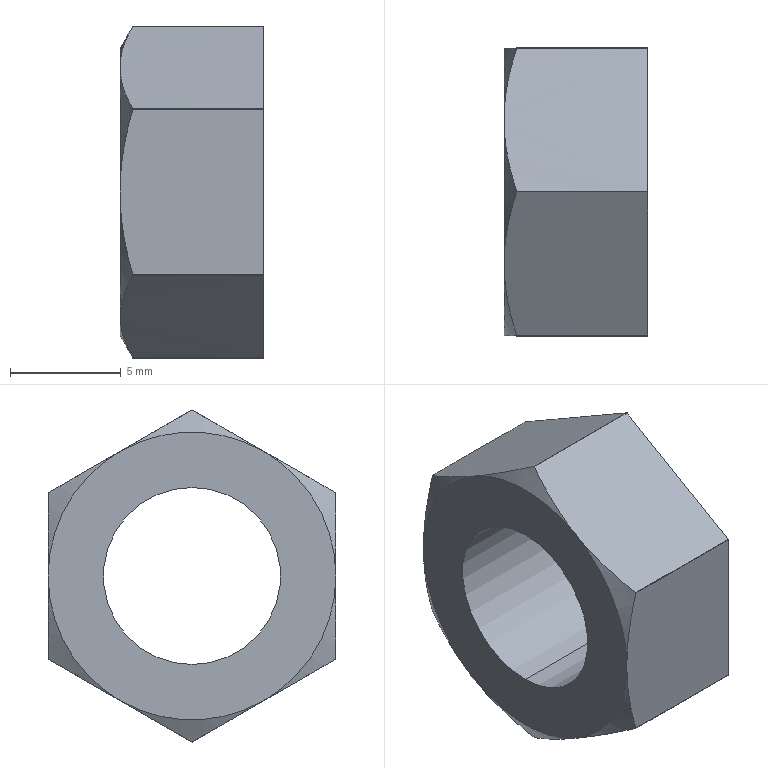Part | STEP file | TNSN20-Y20-F22-Part-12-1 | 1 solid | 22 faces | box 6.5 x 13.002 x 15 mm | volume 622.202 mm3 | cylinder 8 | plane 8 | cone 6 | commonest cylinder face diameters 15 x6 8 x2
STEP:
#1=CARTESIAN_POINT('',(14033.745,13720.046,23.));
#2=VERTEX_POINT('',#1);
#3=CARTESIAN_POINT('',(14033.745,13720.046,15.));
#4=VERTEX_POINT('',#3);
#5=CARTESIAN_POINT('',(14033.745,13720.046,19.));
#6=DIRECTION('',(1.,0.,0.));
#7=DIRECTION('',(0.,1.,0.));
#8=AXIS2_PLACEMENT_3D('',#5,#6,#7);
#9=CIRCLE('',#8,4.);
#10=EDGE_CURVE('',#2,#4,#9,.T.);
#11=ORIENTED_EDGE('',*,*,#10,.T.);
#12=CARTESIAN_POINT('',(14027.245,13720.046,15.));
#13=VERTEX_POINT('',#12);
#14=CARTESIAN_POINT('',(14036.245,13720.046,15.));
#15=DIRECTION('',(-1.,0.,0.));
#16=VECTOR('',#15,1000.);
#17=LINE('',#14,#16);
#18=EDGE_CURVE('',#4,#13,#17,.T.);
#19=ORIENTED_EDGE('',*,*,#18,.T.);
#20=CARTESIAN_POINT('',(14027.245,13720.046,23.));
#21=VERTEX_POINT('',#20);
#22=CARTESIAN_POINT('',(14027.245,13720.046,19.));
#23=DIRECTION('',(1.,0.,0.));
#24=DIRECTION('',(0.,1.,0.));
#25=AXIS2_PLACEMENT_3D('',#22,#23,#24);
#26=CIRCLE('',#25,4.);
#27=EDGE_CURVE('',#21,#13,#26,.T.);
#28=ORIENTED_EDGE('',*,*,#27,.F.);
#29=CARTESIAN_POINT('',(14036.245,13720.046,23.));
#30=DIRECTION('',(-1.,0.,0.));
#31=VECTOR('',#30,1000.);
#32=LINE('',#29,#31);
#33=EDGE_CURVE('',#2,#21,#32,.T.);
#34=ORIENTED_EDGE('',*,*,#33,.F.);
#35=EDGE_LOOP('',(#11,#19,#28,#34));
#36=FACE_OUTER_BOUND('',#35,.T.);
#37=CARTESIAN_POINT('',(14036.245,13720.046,19.));
#38=DIRECTION('',(-1.,0.,0.));
#39=DIRECTION('',(0.,0.,1.));
#40=AXIS2_PLACEMENT_3D('',#37,#38,#39);
#41=CYLINDRICAL_SURFACE('',#40,4.);
#42=ADVANCED_FACE('',(#36),#41,.F.);
#43=CARTESIAN_POINT('',(14027.822,13713.546,15.258));
#44=VERTEX_POINT('',#43);
#45=CARTESIAN_POINT('',(14027.822,13713.556,15.242));
#46=VERTEX_POINT('',#45);
#47=CARTESIAN_POINT('',(14027.822,13720.046,19.));
#48=DIRECTION('',(1.,0.,0.));
#49=DIRECTION('',(0.,-0.8667,-0.4989));
#50=AXIS2_PLACEMENT_3D('',#47,#48,#49);
#51=CIRCLE('',#50,7.5);
#52=EDGE_CURVE('',#44,#46,#51,.T.);
#53=ORIENTED_EDGE('',*,*,#52,.F.);
#54=CARTESIAN_POINT('',(14027.245,13713.546,19.));
#55=VERTEX_POINT('',#54);
#56=CARTESIAN_POINT('',(14027.822,13713.546,15.258));
#57=CARTESIAN_POINT('',(14027.647,13713.551,15.861));
#58=CARTESIAN_POINT('',(14027.502,13713.545,16.485));
#59=CARTESIAN_POINT('',(14027.3,13713.545,17.735));
#60=CARTESIAN_POINT('',(14027.244,13713.549,18.361));
#61=CARTESIAN_POINT('',(14027.245,13713.546,19.));
#62=B_SPLINE_CURVE_WITH_KNOTS('',3,(#56,#57,#58,#59,#60,#61),.UNSPECIFIED.,.F.,.F.,(4,2,4),(0.,0.5,1.),.UNSPECIFIED.);
#63=EDGE_CURVE('',#44,#55,#62,.T.);
#64=ORIENTED_EDGE('',*,*,#63,.T.);
#65=CARTESIAN_POINT('',(14027.245,13716.796,13.371));
#66=VERTEX_POINT('',#65);
#67=CARTESIAN_POINT('',(14027.245,13720.046,19.));
#68=DIRECTION('',(1.,0.,0.));
#69=DIRECTION('',(0.,-1.,0.));
#70=AXIS2_PLACEMENT_3D('',#67,#68,#69);
#71=CIRCLE('',#70,6.5);
#72=EDGE_CURVE('',#55,#66,#71,.T.);
#73=ORIENTED_EDGE('',*,*,#72,.T.);
#74=CARTESIAN_POINT('',(14027.245,13716.796,13.371));
#75=CARTESIAN_POINT('',(14027.244,13716.244,13.692));
#76=CARTESIAN_POINT('',(14027.3,13715.7,14.002));
#77=CARTESIAN_POINT('',(14027.502,13714.618,14.627));
#78=CARTESIAN_POINT('',(14027.647,13714.08,14.944));
#79=CARTESIAN_POINT('',(14027.822,13713.556,15.242));
#80=B_SPLINE_CURVE_WITH_KNOTS('',3,(#74,#75,#76,#77,#78,#79),.UNSPECIFIED.,.F.,.F.,(4,2,4),(0.,0.5,1.),.UNSPECIFIED.);
#81=EDGE_CURVE('',#66,#46,#80,.T.);
#82=ORIENTED_EDGE('',*,*,#81,.T.);
#83=EDGE_LOOP('',(#53,#64,#73,#82));
#84=FACE_OUTER_BOUND('',#83,.T.);
#85=CARTESIAN_POINT('',(14025.076,13720.046,19.));
#86=DIRECTION('',(1.,0.,0.));
#87=DIRECTION('',(0.,1.,0.));
#88=AXIS2_PLACEMENT_3D('',#85,#86,#87);
#89=CONICAL_SURFACE('',#88,2.744,1.047);
#90=ADVANCED_FACE('',(#84),#89,.T.);
#91=CARTESIAN_POINT('',(14027.245,13716.796,24.629));
#92=VERTEX_POINT('',#91);
#93=CARTESIAN_POINT('',(14027.245,13720.046,19.));
#94=DIRECTION('',(1.,0.,0.));
#95=DIRECTION('',(0.,-0.5,0.866));
#96=AXIS2_PLACEMENT_3D('',#93,#94,#95);
#97=CIRCLE('',#96,6.5);
#98=EDGE_CURVE('',#92,#55,#97,.T.);
#99=ORIENTED_EDGE('',*,*,#98,.T.);
#100=CARTESIAN_POINT('',(14027.822,13713.546,22.742));
#101=VERTEX_POINT('',#100);
#102=CARTESIAN_POINT('',(14027.245,13713.546,19.));
#103=CARTESIAN_POINT('',(14027.244,13713.548,19.639));
#104=CARTESIAN_POINT('',(14027.3,13713.545,20.265));
#105=CARTESIAN_POINT('',(14027.502,13713.545,21.515));
#106=CARTESIAN_POINT('',(14027.647,13713.551,22.139));
#107=CARTESIAN_POINT('',(14027.822,13713.546,22.742));
#108=B_SPLINE_CURVE_WITH_KNOTS('',3,(#102,#103,#104,#105,#106,#107),.UNSPECIFIED.,.F.,.F.,(4,2,4),(0.,0.5,1.),.UNSPECIFIED.);
#109=EDGE_CURVE('',#55,#101,#108,.T.);
#110=ORIENTED_EDGE('',*,*,#109,.T.);
#111=CARTESIAN_POINT('',(14027.822,13713.556,22.758));
#112=VERTEX_POINT('',#111);
#113=CARTESIAN_POINT('',(14027.822,13720.046,19.));
#114=DIRECTION('',(1.,0.,0.));
#115=DIRECTION('',(0.,-0.8654,0.5011));
#116=AXIS2_PLACEMENT_3D('',#113,#114,#115);
#117=CIRCLE('',#116,7.5);
#118=EDGE_CURVE('',#112,#101,#117,.T.);
#119=ORIENTED_EDGE('',*,*,#118,.F.);
#120=CARTESIAN_POINT('',(14027.822,13713.556,22.758));
#121=CARTESIAN_POINT('',(14027.647,13714.08,23.056));
#122=CARTESIAN_POINT('',(14027.502,13714.618,23.373));
#123=CARTESIAN_POINT('',(14027.3,13715.7,23.998));
#124=CARTESIAN_POINT('',(14027.244,13716.244,24.308));
#125=CARTESIAN_POINT('',(14027.245,13716.796,24.629));
#126=B_SPLINE_CURVE_WITH_KNOTS('',3,(#120,#121,#122,#123,#124,#125),.UNSPECIFIED.,.F.,.F.,(4,2,4),(0.,0.5,1.),.UNSPECIFIED.);
#127=EDGE_CURVE('',#112,#92,#126,.T.);
#128=ORIENTED_EDGE('',*,*,#127,.T.);
#129=EDGE_LOOP('',(#99,#110,#119,#128));
#130=FACE_OUTER_BOUND('',#129,.T.);
#131=CARTESIAN_POINT('',(14025.076,13720.046,19.));
#132=DIRECTION('',(1.,0.,0.));
#133=DIRECTION('',(0.,1.,0.));
#134=AXIS2_PLACEMENT_3D('',#131,#132,#133);
#135=CONICAL_SURFACE('',#134,2.744,1.047);
#136=ADVANCED_FACE('',(#130),#135,.T.);
#137=CARTESIAN_POINT('',(14027.245,13726.546,19.));
#138=VERTEX_POINT('',#137);
#139=CARTESIAN_POINT('',(14027.245,13723.296,24.629));
#140=VERTEX_POINT('',#139);
#141=CARTESIAN_POINT('',(14027.245,13720.046,19.));
#142=DIRECTION('',(1.,0.,0.));
#143=DIRECTION('',(0.,1.,0.));
#144=AXIS2_PLACEMENT_3D('',#141,#142,#143);
#145=CIRCLE('',#144,6.5);
#146=EDGE_CURVE('',#138,#140,#145,.T.);
#147=ORIENTED_EDGE('',*,*,#146,.T.);
#148=CARTESIAN_POINT('',(14027.822,13726.537,22.758));
#149=VERTEX_POINT('',#148);
#150=CARTESIAN_POINT('',(14027.245,13723.296,24.629));
#151=CARTESIAN_POINT('',(14027.244,13723.849,24.308));
#152=CARTESIAN_POINT('',(14027.3,13724.392,23.998));
#153=CARTESIAN_POINT('',(14027.502,13725.475,23.373));
#154=CARTESIAN_POINT('',(14027.647,13726.013,23.056));
#155=CARTESIAN_POINT('',(14027.822,13726.537,22.758));
#156=B_SPLINE_CURVE_WITH_KNOTS('',3,(#150,#151,#152,#153,#154,#155),.UNSPECIFIED.,.F.,.F.,(4,2,4),(0.,0.5,1.),.UNSPECIFIED.);
#157=EDGE_CURVE('',#140,#149,#156,.T.);
#158=ORIENTED_EDGE('',*,*,#157,.T.);
#159=CARTESIAN_POINT('',(14027.822,13726.546,22.742));
#160=VERTEX_POINT('',#159);
#161=CARTESIAN_POINT('',(14027.822,13720.046,19.));
#162=DIRECTION('',(1.,0.,0.));
#163=DIRECTION('',(0.,0.8667,0.4989));
#164=AXIS2_PLACEMENT_3D('',#161,#162,#163);
#165=CIRCLE('',#164,7.5);
#166=EDGE_CURVE('',#160,#149,#165,.T.);
#167=ORIENTED_EDGE('',*,*,#166,.F.);
#168=CARTESIAN_POINT('',(14027.822,13726.546,22.742));
#169=CARTESIAN_POINT('',(14027.647,13726.542,22.139));
#170=CARTESIAN_POINT('',(14027.502,13726.547,21.515));
#171=CARTESIAN_POINT('',(14027.3,13726.547,20.265));
#172=CARTESIAN_POINT('',(14027.244,13726.544,19.639));
#173=CARTESIAN_POINT('',(14027.245,13726.546,19.));
#174=B_SPLINE_CURVE_WITH_KNOTS('',3,(#168,#169,#170,#171,#172,#173),.UNSPECIFIED.,.F.,.F.,(4,2,4),(0.,0.5,1.),.UNSPECIFIED.);
#175=EDGE_CURVE('',#160,#138,#174,.T.);
#176=ORIENTED_EDGE('',*,*,#175,.T.);
#177=EDGE_LOOP('',(#147,#158,#167,#176));
#178=FACE_OUTER_BOUND('',#177,.T.);
#179=CARTESIAN_POINT('',(14025.076,13720.046,19.));
#180=DIRECTION('',(1.,0.,0.));
#181=DIRECTION('',(0.,-0.8704,-0.4924));
#182=AXIS2_PLACEMENT_3D('',#179,#180,#181);
#183=CONICAL_SURFACE('',#182,2.744,1.047);
#184=ADVANCED_FACE('',(#178),#183,.T.);
#185=CARTESIAN_POINT('',(14027.245,13723.296,13.371));
#186=VERTEX_POINT('',#185);
#187=CARTESIAN_POINT('',(14027.245,13720.046,19.));
#188=DIRECTION('',(1.,0.,0.));
#189=DIRECTION('',(0.,0.5,-0.866));
#190=AXIS2_PLACEMENT_3D('',#187,#188,#189);
#191=CIRCLE('',#190,6.5);
#192=EDGE_CURVE('',#186,#138,#191,.T.);
#193=ORIENTED_EDGE('',*,*,#192,.T.);
#194=CARTESIAN_POINT('',(14027.822,13726.546,15.258));
#195=VERTEX_POINT('',#194);
#196=CARTESIAN_POINT('',(14027.245,13726.546,19.));
#197=CARTESIAN_POINT('',(14027.244,13726.544,18.361));
#198=CARTESIAN_POINT('',(14027.3,13726.547,17.735));
#199=CARTESIAN_POINT('',(14027.502,13726.547,16.485));
#200=CARTESIAN_POINT('',(14027.647,13726.542,15.861));
#201=CARTESIAN_POINT('',(14027.822,13726.546,15.258));
#202=B_SPLINE_CURVE_WITH_KNOTS('',3,(#196,#197,#198,#199,#200,#201),.UNSPECIFIED.,.F.,.F.,(4,2,4),(0.,0.5,1.),.UNSPECIFIED.);
#203=EDGE_CURVE('',#138,#195,#202,.T.);
#204=ORIENTED_EDGE('',*,*,#203,.T.);
#205=CARTESIAN_POINT('',(14027.822,13726.537,15.242));
#206=VERTEX_POINT('',#205);
#207=CARTESIAN_POINT('',(14027.822,13720.046,19.));
#208=DIRECTION('',(1.,0.,0.));
#209=DIRECTION('',(0.,0.8654,-0.5011));
#210=AXIS2_PLACEMENT_3D('',#207,#208,#209);
#211=CIRCLE('',#210,7.5);
#212=EDGE_CURVE('',#206,#195,#211,.T.);
#213=ORIENTED_EDGE('',*,*,#212,.F.);
#214=CARTESIAN_POINT('',(14027.822,13726.537,15.242));
#215=CARTESIAN_POINT('',(14027.647,13726.013,14.944));
#216=CARTESIAN_POINT('',(14027.502,13725.475,14.627));
#217=CARTESIAN_POINT('',(14027.3,13724.392,14.002));
#218=CARTESIAN_POINT('',(14027.244,13723.849,13.692));
#219=CARTESIAN_POINT('',(14027.245,13723.296,13.371));
#220=B_SPLINE_CURVE_WITH_KNOTS('',3,(#214,#215,#216,#217,#218,#219),.UNSPECIFIED.,.F.,.F.,(4,2,4),(0.,0.5,1.),.UNSPECIFIED.);
#221=EDGE_CURVE('',#206,#186,#220,.T.);
#222=ORIENTED_EDGE('',*,*,#221,.T.);
#223=EDGE_LOOP('',(#193,#204,#213,#222));
#224=FACE_OUTER_BOUND('',#223,.T.);
#225=CARTESIAN_POINT('',(14025.076,13720.046,19.));
#226=DIRECTION('',(1.,0.,0.));
#227=DIRECTION('',(0.,-0.866,0.5));
#228=AXIS2_PLACEMENT_3D('',#225,#226,#227);
#229=CONICAL_SURFACE('',#228,2.744,1.047);
#230=ADVANCED_FACE('',(#224),#229,.T.);
#231=CARTESIAN_POINT('',(14027.245,13720.046,19.));
#232=DIRECTION('',(1.,0.,0.));
#233=DIRECTION('',(0.,-0.5,-0.866));
#234=AXIS2_PLACEMENT_3D('',#231,#232,#233);
#235=CIRCLE('',#234,6.5);
#236=EDGE_CURVE('',#66,#186,#235,.T.);
#237=ORIENTED_EDGE('',*,*,#236,.T.);
#238=CARTESIAN_POINT('',(14027.822,13720.056,11.5));
#239=VERTEX_POINT('',#238);
#240=CARTESIAN_POINT('',(14027.245,13723.296,13.371));
#241=CARTESIAN_POINT('',(14027.244,13722.742,13.053));
#242=CARTESIAN_POINT('',(14027.3,13722.202,12.737));
#243=CARTESIAN_POINT('',(14027.502,13721.119,12.112));
#244=CARTESIAN_POINT('',(14027.647,13720.576,11.805));
#245=CARTESIAN_POINT('',(14027.822,13720.056,11.5));
#246=B_SPLINE_CURVE_WITH_KNOTS('',3,(#240,#241,#242,#243,#244,#245),.UNSPECIFIED.,.F.,.F.,(4,2,4),(0.,0.5,1.),.UNSPECIFIED.);
#247=EDGE_CURVE('',#186,#239,#246,.T.);
#248=ORIENTED_EDGE('',*,*,#247,.T.);
#249=CARTESIAN_POINT('',(14027.822,13720.037,11.5));
#250=VERTEX_POINT('',#249);
#251=CARTESIAN_POINT('',(14027.822,13720.046,19.));
#252=DIRECTION('',(1.,0.,0.));
#253=DIRECTION('',(0.,-0.001284,-1.));
#254=AXIS2_PLACEMENT_3D('',#251,#252,#253);
#255=CIRCLE('',#254,7.5);
#256=EDGE_CURVE('',#250,#239,#255,.T.);
#257=ORIENTED_EDGE('',*,*,#256,.F.);
#258=CARTESIAN_POINT('',(14027.822,13720.037,11.5));
#259=CARTESIAN_POINT('',(14027.647,13719.517,11.805));
#260=CARTESIAN_POINT('',(14027.502,13718.974,12.112));
#261=CARTESIAN_POINT('',(14027.3,13717.891,12.737));
#262=CARTESIAN_POINT('',(14027.244,13717.351,13.053));
#263=CARTESIAN_POINT('',(14027.245,13716.796,13.371));
#264=B_SPLINE_CURVE_WITH_KNOTS('',3,(#258,#259,#260,#261,#262,#263),.UNSPECIFIED.,.F.,.F.,(4,2,4),(0.,0.5,1.),.UNSPECIFIED.);
#265=EDGE_CURVE('',#250,#66,#264,.T.);
#266=ORIENTED_EDGE('',*,*,#265,.T.);
#267=EDGE_LOOP('',(#237,#248,#257,#266));
#268=FACE_OUTER_BOUND('',#267,.T.);
#269=CARTESIAN_POINT('',(14024.977,13720.046,19.));
#270=DIRECTION('',(1.,0.,0.));
#271=DIRECTION('',(0.,1.,0.));
#272=AXIS2_PLACEMENT_3D('',#269,#270,#271);
#273=CONICAL_SURFACE('',#272,2.572,1.047);
#274=ADVANCED_FACE('',(#268),#273,.T.);
#275=ORIENTED_EDGE('',*,*,#118,.T.);
#276=CARTESIAN_POINT('',(14033.745,13713.546,22.742));
#277=VERTEX_POINT('',#276);
#278=CARTESIAN_POINT('',(14027.822,13713.546,22.742));
#279=DIRECTION('',(1.,0.,0.));
#280=VECTOR('',#279,1000.);
#281=LINE('',#278,#280);
#282=EDGE_CURVE('',#101,#277,#281,.T.);
#283=ORIENTED_EDGE('',*,*,#282,.T.);
#284=CARTESIAN_POINT('',(14033.745,13713.556,22.758));
#285=VERTEX_POINT('',#284);
#286=CARTESIAN_POINT('',(14033.745,13720.046,19.));
#287=DIRECTION('',(1.,0.,0.));
#288=DIRECTION('',(0.,-0.8654,0.5011));
#289=AXIS2_PLACEMENT_3D('',#286,#287,#288);
#290=CIRCLE('',#289,7.5);
#291=EDGE_CURVE('',#285,#277,#290,.T.);
#292=ORIENTED_EDGE('',*,*,#291,.F.);
#293=CARTESIAN_POINT('',(14027.822,13713.556,22.758));
#294=DIRECTION('',(1.,0.,0.));
#295=VECTOR('',#294,1000.);
#296=LINE('',#293,#295);
#297=EDGE_CURVE('',#112,#285,#296,.T.);
#298=ORIENTED_EDGE('',*,*,#297,.F.);
#299=EDGE_LOOP('',(#275,#283,#292,#298));
#300=FACE_OUTER_BOUND('',#299,.T.);
#301=CARTESIAN_POINT('',(14030.784,13720.046,19.));
#302=DIRECTION('',(1.,0.,0.));
#303=DIRECTION('',(0.,1.,0.));
#304=AXIS2_PLACEMENT_3D('',#301,#302,#303);
#305=CYLINDRICAL_SURFACE('',#304,7.5);
#306=ADVANCED_FACE('',(#300),#305,.T.);
#307=ORIENTED_EDGE('',*,*,#166,.T.);
#308=CARTESIAN_POINT('',(14033.745,13726.537,22.758));
#309=VERTEX_POINT('',#308);
#310=CARTESIAN_POINT('',(14027.822,13726.537,22.758));
#311=DIRECTION('',(1.,0.,0.));
#312=VECTOR('',#311,1000.);
#313=LINE('',#310,#312);
#314=EDGE_CURVE('',#149,#309,#313,.T.);
#315=ORIENTED_EDGE('',*,*,#314,.T.);
#316=CARTESIAN_POINT('',(14033.745,13726.546,22.742));
#317=VERTEX_POINT('',#316);
#318=CARTESIAN_POINT('',(14033.745,13720.046,19.));
#319=DIRECTION('',(1.,0.,0.));
#320=DIRECTION('',(0.,0.8667,0.4989));
#321=AXIS2_PLACEMENT_3D('',#318,#319,#320);
#322=CIRCLE('',#321,7.5);
#323=EDGE_CURVE('',#317,#309,#322,.T.);
#324=ORIENTED_EDGE('',*,*,#323,.F.);
#325=CARTESIAN_POINT('',(14027.822,13726.546,22.742));
#326=DIRECTION('',(1.,0.,0.));
#327=VECTOR('',#326,1000.);
#328=LINE('',#325,#327);
#329=EDGE_CURVE('',#160,#317,#328,.T.);
#330=ORIENTED_EDGE('',*,*,#329,.F.);
#331=EDGE_LOOP('',(#307,#315,#324,#330));
#332=FACE_OUTER_BOUND('',#331,.T.);
#333=CARTESIAN_POINT('',(14030.784,13720.046,19.));
#334=DIRECTION('',(1.,0.,0.));
#335=DIRECTION('',(0.,1.,0.));
#336=AXIS2_PLACEMENT_3D('',#333,#334,#335);
#337=CYLINDRICAL_SURFACE('',#336,7.5);
#338=ADVANCED_FACE('',(#332),#337,.T.);
#339=ORIENTED_EDGE('',*,*,#212,.T.);
#340=CARTESIAN_POINT('',(14033.745,13726.546,15.258));
#341=VERTEX_POINT('',#340);
#342=CARTESIAN_POINT('',(14027.822,13726.546,15.258));
#343=DIRECTION('',(1.,0.,0.));
#344=VECTOR('',#343,1000.);
#345=LINE('',#342,#344);
#346=EDGE_CURVE('',#195,#341,#345,.T.);
#347=ORIENTED_EDGE('',*,*,#346,.T.);
#348=CARTESIAN_POINT('',(14033.745,13726.537,15.242));
#349=VERTEX_POINT('',#348);
#350=CARTESIAN_POINT('',(14033.745,13720.046,19.));
#351=DIRECTION('',(1.,0.,0.));
#352=DIRECTION('',(0.,0.8654,-0.5011));
#353=AXIS2_PLACEMENT_3D('',#350,#351,#352);
#354=CIRCLE('',#353,7.5);
#355=EDGE_CURVE('',#349,#341,#354,.T.);
#356=ORIENTED_EDGE('',*,*,#355,.F.);
#357=CARTESIAN_POINT('',(14027.822,13726.537,15.242));
#358=DIRECTION('',(1.,0.,0.));
#359=VECTOR('',#358,1000.);
#360=LINE('',#357,#359);
#361=EDGE_CURVE('',#206,#349,#360,.T.);
#362=ORIENTED_EDGE('',*,*,#361,.F.);
#363=EDGE_LOOP('',(#339,#347,#356,#362));
#364=FACE_OUTER_BOUND('',#363,.T.);
#365=CARTESIAN_POINT('',(14030.784,13720.046,19.));
#366=DIRECTION('',(1.,0.,0.));
#367=DIRECTION('',(0.,1.,0.));
#368=AXIS2_PLACEMENT_3D('',#365,#366,#367);
#369=CYLINDRICAL_SURFACE('',#368,7.5);
#370=ADVANCED_FACE('',(#364),#369,.T.);
#371=ORIENTED_EDGE('',*,*,#256,.T.);
#372=CARTESIAN_POINT('',(14033.745,13720.056,11.5));
#373=VERTEX_POINT('',#372);
#374=CARTESIAN_POINT('',(14027.822,13720.056,11.5));
#375=DIRECTION('',(1.,0.,0.));
#376=VECTOR('',#375,1000.);
#377=LINE('',#374,#376);
#378=EDGE_CURVE('',#239,#373,#377,.T.);
#379=ORIENTED_EDGE('',*,*,#378,.T.);
#380=CARTESIAN_POINT('',(14033.745,13720.037,11.5));
#381=VERTEX_POINT('',#380);
#382=CARTESIAN_POINT('',(14033.745,13720.046,19.));
#383=DIRECTION('',(1.,0.,0.));
#384=DIRECTION('',(0.,-0.001284,-1.));
#385=AXIS2_PLACEMENT_3D('',#382,#383,#384);
#386=CIRCLE('',#385,7.5);
#387=EDGE_CURVE('',#381,#373,#386,.T.);
#388=ORIENTED_EDGE('',*,*,#387,.F.);
#389=CARTESIAN_POINT('',(14027.822,13720.037,11.5));
#390=DIRECTION('',(1.,0.,0.));
#391=VECTOR('',#390,1000.);
#392=LINE('',#389,#391);
#393=EDGE_CURVE('',#250,#381,#392,.T.);
#394=ORIENTED_EDGE('',*,*,#393,.F.);
#395=EDGE_LOOP('',(#371,#379,#388,#394));
#396=FACE_OUTER_BOUND('',#395,.T.);
#397=CARTESIAN_POINT('',(14030.784,13720.046,19.));
#398=DIRECTION('',(1.,0.,0.));
#399=DIRECTION('',(0.,1.,0.));
#400=AXIS2_PLACEMENT_3D('',#397,#398,#399);
#401=CYLINDRICAL_SURFACE('',#400,7.5);
#402=ADVANCED_FACE('',(#396),#401,.T.);
#403=CARTESIAN_POINT('',(14033.745,13713.546,15.258));
#404=VERTEX_POINT('',#403);
#405=CARTESIAN_POINT('',(14033.745,13713.556,15.242));
#406=VERTEX_POINT('',#405);
#407=CARTESIAN_POINT('',(14033.745,13720.046,19.));
#408=DIRECTION('',(1.,0.,0.));
#409=DIRECTION('',(0.,-0.8667,-0.4989));
#410=AXIS2_PLACEMENT_3D('',#407,#408,#409);
#411=CIRCLE('',#410,7.5);
#412=EDGE_CURVE('',#404,#406,#411,.T.);
#413=ORIENTED_EDGE('',*,*,#412,.F.);
#414=CARTESIAN_POINT('',(14027.822,13713.546,15.258));
#415=DIRECTION('',(1.,0.,0.));
#416=VECTOR('',#415,1000.);
#417=LINE('',#414,#416);
#418=EDGE_CURVE('',#44,#404,#417,.T.);
#419=ORIENTED_EDGE('',*,*,#418,.F.);
#420=ORIENTED_EDGE('',*,*,#52,.T.);
#421=CARTESIAN_POINT('',(14027.822,13713.556,15.242));
#422=DIRECTION('',(1.,0.,0.));
#423=VECTOR('',#422,1000.);
#424=LINE('',#421,#423);
#425=EDGE_CURVE('',#46,#406,#424,.T.);
#426=ORIENTED_EDGE('',*,*,#425,.T.);
#427=EDGE_LOOP('',(#413,#419,#420,#426));
#428=FACE_OUTER_BOUND('',#427,.T.);
#429=CARTESIAN_POINT('',(14030.784,13720.046,19.));
#430=DIRECTION('',(1.,0.,0.));
#431=DIRECTION('',(0.,1.,0.));
#432=AXIS2_PLACEMENT_3D('',#429,#430,#431);
#433=CYLINDRICAL_SURFACE('',#432,7.5);
#434=ADVANCED_FACE('',(#428),#433,.T.);
#435=CARTESIAN_POINT('',(14027.245,13720.046,19.));
#436=DIRECTION('',(1.,0.,0.));
#437=DIRECTION('',(0.,0.5,0.866));
#438=AXIS2_PLACEMENT_3D('',#435,#436,#437);
#439=CIRCLE('',#438,6.5);
#440=EDGE_CURVE('',#140,#92,#439,.T.);
#441=ORIENTED_EDGE('',*,*,#440,.F.);
#442=ORIENTED_EDGE('',*,*,#146,.F.);
#443=ORIENTED_EDGE('',*,*,#192,.F.);
#444=ORIENTED_EDGE('',*,*,#236,.F.);
#445=ORIENTED_EDGE('',*,*,#72,.F.);
#446=ORIENTED_EDGE('',*,*,#98,.F.);
#447=EDGE_LOOP('',(#441,#442,#443,#444,#445,#446));
#448=FACE_OUTER_BOUND('',#447,.T.);
#449=ORIENTED_EDGE('',*,*,#27,.T.);
#450=CARTESIAN_POINT('',(14027.245,13720.046,19.));
#451=DIRECTION('',(1.,0.,0.));
#452=DIRECTION('',(0.,1.,0.));
#453=AXIS2_PLACEMENT_3D('',#450,#451,#452);
#454=CIRCLE('',#453,4.);
#455=EDGE_CURVE('',#13,#21,#454,.T.);
#456=ORIENTED_EDGE('',*,*,#455,.T.);
#457=EDGE_LOOP('',(#449,#456));
#458=FACE_BOUND('',#457,.T.);
#459=CARTESIAN_POINT('',(14027.245,13703.643,3.347));
#460=DIRECTION('',(1.,0.,0.));
#461=DIRECTION('',(0.,1.,0.));
#462=AXIS2_PLACEMENT_3D('',#459,#460,#461);
#463=PLANE('',#462);
#464=ADVANCED_FACE('',(#448,#458),#463,.F.);
#465=ORIENTED_EDGE('',*,*,#440,.T.);
#466=CARTESIAN_POINT('',(14027.822,13720.037,26.5));
#467=VERTEX_POINT('',#466);
#468=CARTESIAN_POINT('',(14027.245,13716.796,24.629));
#469=CARTESIAN_POINT('',(14027.244,13717.351,24.947));
#470=CARTESIAN_POINT('',(14027.3,13717.891,25.263));
#471=CARTESIAN_POINT('',(14027.502,13718.974,25.888));
#472=CARTESIAN_POINT('',(14027.647,13719.517,26.195));
#473=CARTESIAN_POINT('',(14027.822,13720.037,26.5));
#474=B_SPLINE_CURVE_WITH_KNOTS('',3,(#468,#469,#470,#471,#472,#473),.UNSPECIFIED.,.F.,.F.,(4,2,4),(0.,0.5,1.),.UNSPECIFIED.);
#475=EDGE_CURVE('',#92,#467,#474,.T.);
#476=ORIENTED_EDGE('',*,*,#475,.T.);
#477=CARTESIAN_POINT('',(14027.822,13720.056,26.5));
#478=VERTEX_POINT('',#477);
#479=CARTESIAN_POINT('',(14027.822,13720.046,19.));
#480=DIRECTION('',(1.,0.,0.));
#481=DIRECTION('',(0.,0.001284,1.));
#482=AXIS2_PLACEMENT_3D('',#479,#480,#481);
#483=CIRCLE('',#482,7.5);
#484=EDGE_CURVE('',#478,#467,#483,.T.);
#485=ORIENTED_EDGE('',*,*,#484,.F.);
#486=CARTESIAN_POINT('',(14027.822,13720.056,26.5));
#487=CARTESIAN_POINT('',(14027.647,13720.576,26.195));
#488=CARTESIAN_POINT('',(14027.502,13721.119,25.888));
#489=CARTESIAN_POINT('',(14027.3,13722.201,25.263));
#490=CARTESIAN_POINT('',(14027.244,13722.742,24.947));
#491=CARTESIAN_POINT('',(14027.245,13723.296,24.629));
#492=B_SPLINE_CURVE_WITH_KNOTS('',3,(#486,#487,#488,#489,#490,#491),.UNSPECIFIED.,.F.,.F.,(4,2,4),(0.,0.5,1.),.UNSPECIFIED.);
#493=EDGE_CURVE('',#478,#140,#492,.T.);
#494=ORIENTED_EDGE('',*,*,#493,.T.);
#495=EDGE_LOOP('',(#465,#476,#485,#494));
#496=FACE_OUTER_BOUND('',#495,.T.);
#497=CARTESIAN_POINT('',(14024.977,13720.046,19.));
#498=DIRECTION('',(1.,0.,0.));
#499=DIRECTION('',(0.,1.,0.));
#500=AXIS2_PLACEMENT_3D('',#497,#498,#499);
#501=CONICAL_SURFACE('',#500,2.572,1.047);
#502=ADVANCED_FACE('',(#496),#501,.T.);
#503=CARTESIAN_POINT('',(14033.745,13720.056,26.5));
#504=VERTEX_POINT('',#503);
#505=CARTESIAN_POINT('',(14033.745,13720.037,26.5));
#506=VERTEX_POINT('',#505);
#507=CARTESIAN_POINT('',(14033.745,13720.046,19.));
#508=DIRECTION('',(1.,0.,0.));
#509=DIRECTION('',(0.,0.001284,1.));
#510=AXIS2_PLACEMENT_3D('',#507,#508,#509);
#511=CIRCLE('',#510,7.5);
#512=EDGE_CURVE('',#504,#506,#511,.T.);
#513=ORIENTED_EDGE('',*,*,#512,.F.);
#514=CARTESIAN_POINT('',(14027.822,13720.056,26.5));
#515=DIRECTION('',(1.,0.,0.));
#516=VECTOR('',#515,1000.);
#517=LINE('',#514,#516);
#518=EDGE_CURVE('',#478,#504,#517,.T.);
#519=ORIENTED_EDGE('',*,*,#518,.F.);
#520=ORIENTED_EDGE('',*,*,#484,.T.);
#521=CARTESIAN_POINT('',(14027.822,13720.037,26.5));
#522=DIRECTION('',(1.,0.,0.));
#523=VECTOR('',#522,1000.);
#524=LINE('',#521,#523);
#525=EDGE_CURVE('',#467,#506,#524,.T.);
#526=ORIENTED_EDGE('',*,*,#525,.T.);
#527=EDGE_LOOP('',(#513,#519,#520,#526));
#528=FACE_OUTER_BOUND('',#527,.T.);
#529=CARTESIAN_POINT('',(14030.784,13720.046,19.));
#530=DIRECTION('',(1.,0.,0.));
#531=DIRECTION('',(0.,1.,0.));
#532=AXIS2_PLACEMENT_3D('',#529,#530,#531);
#533=CYLINDRICAL_SURFACE('',#532,7.5);
#534=ADVANCED_FACE('',(#528),#533,.T.);
#535=ORIENTED_EDGE('',*,*,#291,.T.);
#536=CARTESIAN_POINT('',(14033.745,13713.546,22.742));
#537=DIRECTION('',(0.,0.,-1.));
#538=VECTOR('',#537,1000.);
#539=LINE('',#536,#538);
#540=EDGE_CURVE('',#277,#404,#539,.T.);
#541=ORIENTED_EDGE('',*,*,#540,.T.);
#542=ORIENTED_EDGE('',*,*,#412,.T.);
#543=CARTESIAN_POINT('',(14033.745,13713.556,15.242));
#544=DIRECTION('',(0.,0.866,-0.5));
#545=VECTOR('',#544,1000.);
#546=LINE('',#543,#545);
#547=EDGE_CURVE('',#406,#381,#546,.T.);
#548=ORIENTED_EDGE('',*,*,#547,.T.);
#549=ORIENTED_EDGE('',*,*,#387,.T.);
#550=CARTESIAN_POINT('',(14033.745,13720.056,11.5));
#551=DIRECTION('',(0.,0.866,0.5));
#552=VECTOR('',#551,1000.);
#553=LINE('',#550,#552);
#554=EDGE_CURVE('',#373,#349,#553,.T.);
#555=ORIENTED_EDGE('',*,*,#554,.T.);
#556=ORIENTED_EDGE('',*,*,#355,.T.);
#557=CARTESIAN_POINT('',(14033.745,13726.546,15.258));
#558=DIRECTION('',(0.,0.,1.));
#559=VECTOR('',#558,1000.);
#560=LINE('',#557,#559);
#561=EDGE_CURVE('',#341,#317,#560,.T.);
#562=ORIENTED_EDGE('',*,*,#561,.T.);
#563=ORIENTED_EDGE('',*,*,#323,.T.);
#564=CARTESIAN_POINT('',(14033.745,13726.537,22.758));
#565=DIRECTION('',(0.,-0.866,0.5));
#566=VECTOR('',#565,1000.);
#567=LINE('',#564,#566);
#568=EDGE_CURVE('',#309,#504,#567,.T.);
#569=ORIENTED_EDGE('',*,*,#568,.T.);
#570=ORIENTED_EDGE('',*,*,#512,.T.);
#571=CARTESIAN_POINT('',(14033.745,13720.037,26.5));
#572=DIRECTION('',(0.,-0.866,-0.5));
#573=VECTOR('',#572,1000.);
#574=LINE('',#571,#573);
#575=EDGE_CURVE('',#506,#285,#574,.T.);
#576=ORIENTED_EDGE('',*,*,#575,.T.);
#577=EDGE_LOOP('',(#535,#541,#542,#548,#549,#555,#556,#562,#563,#569,#570,#576));
#578=FACE_OUTER_BOUND('',#577,.T.);
#579=ORIENTED_EDGE('',*,*,#10,.F.);
#580=CARTESIAN_POINT('',(14033.745,13720.046,19.));
#581=DIRECTION('',(1.,0.,0.));
#582=DIRECTION('',(0.,1.,0.));
#583=AXIS2_PLACEMENT_3D('',#580,#581,#582);
#584=CIRCLE('',#583,4.);
#585=EDGE_CURVE('',#4,#2,#584,.T.);
#586=ORIENTED_EDGE('',*,*,#585,.F.);
#587=EDGE_LOOP('',(#579,#586));
#588=FACE_BOUND('',#587,.T.);
#589=CARTESIAN_POINT('',(14033.745,13734.943,3.353));
#590=DIRECTION('',(-1.,0.,0.));
#591=DIRECTION('',(0.,-1.,0.));
#592=AXIS2_PLACEMENT_3D('',#589,#590,#591);
#593=PLANE('',#592);
#594=ADVANCED_FACE('',(#578,#588),#593,.F.);
#595=ORIENTED_EDGE('',*,*,#81,.F.);
#596=ORIENTED_EDGE('',*,*,#265,.F.);
#597=ORIENTED_EDGE('',*,*,#393,.T.);
#598=ORIENTED_EDGE('',*,*,#547,.F.);
#599=ORIENTED_EDGE('',*,*,#425,.F.);
#600=EDGE_LOOP('',(#595,#596,#597,#598,#599));
#601=FACE_OUTER_BOUND('',#600,.T.);
#602=CARTESIAN_POINT('',(14023.061,13723.234,9.654));
#603=DIRECTION('',(0.,0.5,0.866));
#604=DIRECTION('',(0.,-0.866,0.5));
#605=AXIS2_PLACEMENT_3D('',#602,#603,#604);
#606=PLANE('',#605);
#607=ADVANCED_FACE('',(#601),#606,.F.);
#608=ORIENTED_EDGE('',*,*,#247,.F.);
#609=ORIENTED_EDGE('',*,*,#221,.F.);
#610=ORIENTED_EDGE('',*,*,#361,.T.);
#611=ORIENTED_EDGE('',*,*,#554,.F.);
#612=ORIENTED_EDGE('',*,*,#378,.F.);
#613=EDGE_LOOP('',(#608,#609,#610,#611,#612));
#614=FACE_OUTER_BOUND('',#613,.T.);
#615=CARTESIAN_POINT('',(14023.061,13729.734,17.088));
#616=DIRECTION('',(0.,-0.5,0.866));
#617=DIRECTION('',(0.,-0.866,-0.5));
#618=AXIS2_PLACEMENT_3D('',#615,#616,#617);
#619=PLANE('',#618);
#620=ADVANCED_FACE('',(#614),#619,.F.);
#621=ORIENTED_EDGE('',*,*,#203,.F.);
#622=ORIENTED_EDGE('',*,*,#175,.F.);
#623=ORIENTED_EDGE('',*,*,#329,.T.);
#624=ORIENTED_EDGE('',*,*,#561,.F.);
#625=ORIENTED_EDGE('',*,*,#346,.F.);
#626=EDGE_LOOP('',(#621,#622,#623,#624,#625));
#627=FACE_OUTER_BOUND('',#626,.T.);
#628=CARTESIAN_POINT('',(14023.061,13726.546,11.566));
#629=DIRECTION('',(0.,-1.,0.));
#630=DIRECTION('',(1.,0.,0.));
#631=AXIS2_PLACEMENT_3D('',#628,#629,#630);
#632=PLANE('',#631);
#633=ADVANCED_FACE('',(#627),#632,.F.);
#634=ORIENTED_EDGE('',*,*,#157,.F.);
#635=ORIENTED_EDGE('',*,*,#493,.F.);
#636=ORIENTED_EDGE('',*,*,#518,.T.);
#637=ORIENTED_EDGE('',*,*,#568,.F.);
#638=ORIENTED_EDGE('',*,*,#314,.F.);
#639=EDGE_LOOP('',(#634,#635,#636,#637,#638));
#640=FACE_OUTER_BOUND('',#639,.T.);
#641=CARTESIAN_POINT('',(14023.061,13716.858,28.346));
#642=DIRECTION('',(0.,-0.5,-0.866));
#643=DIRECTION('',(0.,0.866,-0.5));
#644=AXIS2_PLACEMENT_3D('',#641,#642,#643);
#645=PLANE('',#644);
#646=ADVANCED_FACE('',(#640),#645,.F.);
#647=ORIENTED_EDGE('',*,*,#475,.F.);
#648=ORIENTED_EDGE('',*,*,#127,.F.);
#649=ORIENTED_EDGE('',*,*,#297,.T.);
#650=ORIENTED_EDGE('',*,*,#575,.F.);
#651=ORIENTED_EDGE('',*,*,#525,.F.);
#652=EDGE_LOOP('',(#647,#648,#649,#650,#651));
#653=FACE_OUTER_BOUND('',#652,.T.);
#654=CARTESIAN_POINT('',(14023.061,13710.358,20.912));
#655=DIRECTION('',(0.,0.5,-0.866));
#656=DIRECTION('',(0.,0.866,0.5));
#657=AXIS2_PLACEMENT_3D('',#654,#655,#656);
#658=PLANE('',#657);
#659=ADVANCED_FACE('',(#653),#658,.F.);
#660=ORIENTED_EDGE('',*,*,#109,.F.);
#661=ORIENTED_EDGE('',*,*,#63,.F.);
#662=ORIENTED_EDGE('',*,*,#418,.T.);
#663=ORIENTED_EDGE('',*,*,#540,.F.);
#664=ORIENTED_EDGE('',*,*,#282,.F.);
#665=EDGE_LOOP('',(#660,#661,#662,#663,#664));
#666=FACE_OUTER_BOUND('',#665,.T.);
#667=CARTESIAN_POINT('',(14037.929,13713.546,11.566));
#668=DIRECTION('',(0.,1.,0.));
#669=DIRECTION('',(-1.,0.,0.));
#670=AXIS2_PLACEMENT_3D('',#667,#668,#669);
#671=PLANE('',#670);
#672=ADVANCED_FACE('',(#666),#671,.F.);
#673=ORIENTED_EDGE('',*,*,#18,.F.);
#674=ORIENTED_EDGE('',*,*,#585,.T.);
#675=ORIENTED_EDGE('',*,*,#33,.T.);
#676=ORIENTED_EDGE('',*,*,#455,.F.);
#677=EDGE_LOOP('',(#673,#674,#675,#676));
#678=FACE_OUTER_BOUND('',#677,.T.);
#679=CARTESIAN_POINT('',(14036.245,13720.046,19.));
#680=DIRECTION('',(-1.,0.,0.));
#681=DIRECTION('',(0.,0.,1.));
#682=AXIS2_PLACEMENT_3D('',#679,#680,#681);
#683=CYLINDRICAL_SURFACE('',#682,4.);
#684=ADVANCED_FACE('',(#678),#683,.F.);
#685=CLOSED_SHELL('',(#42,#90,#136,#184,#230,#274,#306,#338,#370,#402,#434,#464,#502,#534,#594,#607,#620,#633,#646,#659,#672,#684));
#686=MANIFOLD_SOLID_BREP('',#685);
#687=CARTESIAN_POINT('',(0.,0.,0.));
#688=DIRECTION('',(0.,0.,1.));
#689=DIRECTION('',(1.,0.,0.));
#690=AXIS2_PLACEMENT_3D('',#687,#688,#689);
#691=(LENGTH_UNIT()NAMED_UNIT(*)SI_UNIT(.MILLI.,.METRE.));
#692=UNCERTAINTY_MEASURE_WITH_UNIT(LENGTH_MEASURE(0.00001),#691,'','');
#693=(NAMED_UNIT(*)PLANE_ANGLE_UNIT()SI_UNIT($,.RADIAN.));
#694=(NAMED_UNIT(*)SI_UNIT($,.STERADIAN.)SOLID_ANGLE_UNIT());
#695=(GEOMETRIC_REPRESENTATION_CONTEXT(3)GLOBAL_UNCERTAINTY_ASSIGNED_CONTEXT((#692))GLOBAL_UNIT_ASSIGNED_CONTEXT((#691,#693,#694))REPRESENTATION_CONTEXT('',''));
#696=ADVANCED_BREP_SHAPE_REPRESENTATION('',(#686,#690),#695);